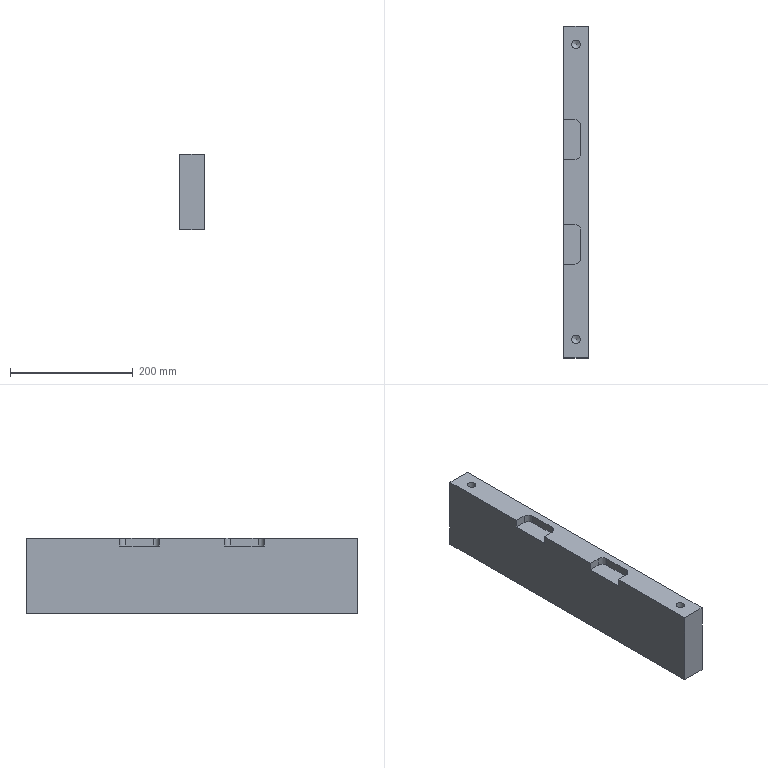Part | NX | features LIN_SOLID_COLOR 2 | 1 solid | 22 faces | box 40 x 540 x 123.5 mm | volume 2609030 mm3 | plane 14 | cylinder 6 | cone 2 | commonest cylinder face diameters 20 x4 14 x2
STEP:
#1=CARTESIAN_POINT('',(606.,270.,-106.5));
#2=VERTEX_POINT('',#1);
#3=CARTESIAN_POINT('',(566.,270.,-106.5));
#4=VERTEX_POINT('',#3);
#5=CARTESIAN_POINT('',(-164.,270.,-106.5));
#6=DIRECTION('',(1.,0.,0.));
#7=VECTOR('',#6,1000.);
#8=LINE('',#5,#7);
#9=EDGE_CURVE('',#2,#4,#8,.F.);
#10=ORIENTED_EDGE('',*,*,#9,.F.);
#11=CARTESIAN_POINT('',(606.,270.,-230.));
#12=VERTEX_POINT('',#11);
#13=CARTESIAN_POINT('',(606.,270.,-111.5));
#14=DIRECTION('',(0.,0.,-1.));
#15=VECTOR('',#14,1000.);
#16=LINE('',#13,#15);
#17=EDGE_CURVE('',#12,#2,#16,.F.);
#18=ORIENTED_EDGE('',*,*,#17,.F.);
#19=CARTESIAN_POINT('',(566.,270.,-230.));
#20=VERTEX_POINT('',#19);
#21=CARTESIAN_POINT('',(426.,270.,-230.));
#22=DIRECTION('',(1.,0.,0.));
#23=VECTOR('',#22,1000.);
#24=LINE('',#21,#23);
#25=EDGE_CURVE('',#12,#20,#24,.F.);
#26=ORIENTED_EDGE('',*,*,#25,.T.);
#27=CARTESIAN_POINT('',(566.,270.,-111.5));
#28=DIRECTION('',(0.,0.,-1.));
#29=VECTOR('',#28,1000.);
#30=LINE('',#27,#29);
#31=EDGE_CURVE('',#20,#4,#30,.F.);
#32=ORIENTED_EDGE('',*,*,#31,.T.);
#33=EDGE_LOOP('',(#10,#18,#26,#32));
#34=FACE_BOUND('',#33,.T.);
#35=CARTESIAN_POINT('',(426.,270.,-111.5));
#36=DIRECTION('',(0.,1.,0.));
#37=DIRECTION('',(0.,0.,1.));
#38=AXIS2_PLACEMENT_3D('',#35,#36,#37);
#39=PLANE('',#38);
#40=ADVANCED_FACE('',(#34),#39,.T.);
#41=CARTESIAN_POINT('',(566.,-270.,-230.));
#42=VERTEX_POINT('',#41);
#43=CARTESIAN_POINT('',(566.,0.,-230.));
#44=DIRECTION('',(0.,-1.,0.));
#45=VECTOR('',#44,1000.);
#46=LINE('',#43,#45);
#47=EDGE_CURVE('',#20,#42,#46,.T.);
#48=ORIENTED_EDGE('',*,*,#47,.F.);
#49=ORIENTED_EDGE('',*,*,#25,.F.);
#50=CARTESIAN_POINT('',(606.,-270.,-230.));
#51=VERTEX_POINT('',#50);
#52=CARTESIAN_POINT('',(606.,0.,-230.));
#53=DIRECTION('',(0.,-1.,0.));
#54=VECTOR('',#53,1000.);
#55=LINE('',#52,#54);
#56=EDGE_CURVE('',#12,#51,#55,.T.);
#57=ORIENTED_EDGE('',*,*,#56,.T.);
#58=CARTESIAN_POINT('',(426.,-270.,-230.));
#59=DIRECTION('',(1.,0.,0.));
#60=VECTOR('',#59,1000.);
#61=LINE('',#58,#60);
#62=EDGE_CURVE('',#51,#42,#61,.F.);
#63=ORIENTED_EDGE('',*,*,#62,.T.);
#64=EDGE_LOOP('',(#48,#49,#57,#63));
#65=FACE_BOUND('',#64,.T.);
#66=CARTESIAN_POINT('',(426.,0.,-230.));
#67=DIRECTION('',(0.,0.,1.));
#68=DIRECTION('',(-1.,0.,0.));
#69=AXIS2_PLACEMENT_3D('',#66,#67,#68);
#70=PLANE('',#69);
#71=ADVANCED_FACE('',(#65),#70,.F.);
#72=ORIENTED_EDGE('',*,*,#62,.F.);
#73=CARTESIAN_POINT('',(606.,-270.,-106.5));
#74=VERTEX_POINT('',#73);
#75=CARTESIAN_POINT('',(606.,-270.,-101.5));
#76=DIRECTION('',(0.,0.,-1.));
#77=VECTOR('',#76,1000.);
#78=LINE('',#75,#77);
#79=EDGE_CURVE('',#51,#74,#78,.F.);
#80=ORIENTED_EDGE('',*,*,#79,.T.);
#81=CARTESIAN_POINT('',(566.,-270.,-106.5));
#82=VERTEX_POINT('',#81);
#83=CARTESIAN_POINT('',(426.,-270.,-106.5));
#84=DIRECTION('',(1.,0.,0.));
#85=VECTOR('',#84,1000.);
#86=LINE('',#83,#85);
#87=EDGE_CURVE('',#74,#82,#86,.F.);
#88=ORIENTED_EDGE('',*,*,#87,.T.);
#89=CARTESIAN_POINT('',(566.,-270.,-101.5));
#90=DIRECTION('',(0.,0.,-1.));
#91=VECTOR('',#90,1000.);
#92=LINE('',#89,#91);
#93=EDGE_CURVE('',#42,#82,#92,.F.);
#94=ORIENTED_EDGE('',*,*,#93,.F.);
#95=EDGE_LOOP('',(#72,#80,#88,#94));
#96=FACE_BOUND('',#95,.T.);
#97=CARTESIAN_POINT('',(426.,-270.,-111.5));
#98=DIRECTION('',(0.,-1.,0.));
#99=DIRECTION('',(0.,0.,-1.));
#100=AXIS2_PLACEMENT_3D('',#97,#98,#99);
#101=PLANE('',#100);
#102=ADVANCED_FACE('',(#96),#101,.T.);
#103=CARTESIAN_POINT('',(566.,117.5,-106.5));
#104=VERTEX_POINT('',#103);
#105=CARTESIAN_POINT('',(566.,0.,-106.5));
#106=DIRECTION('',(0.,1.,0.));
#107=VECTOR('',#106,1000.);
#108=LINE('',#105,#107);
#109=EDGE_CURVE('',#104,#4,#108,.T.);
#110=ORIENTED_EDGE('',*,*,#109,.F.);
#111=CARTESIAN_POINT('',(584.,117.5,-106.5));
#112=VERTEX_POINT('',#111);
#113=CARTESIAN_POINT('',(-164.,117.5,-106.5));
#114=DIRECTION('',(1.,0.,0.));
#115=VECTOR('',#114,1000.);
#116=LINE('',#113,#115);
#117=EDGE_CURVE('',#104,#112,#116,.T.);
#118=ORIENTED_EDGE('',*,*,#117,.T.);
#119=CARTESIAN_POINT('',(594.,107.5,-106.5));
#120=VERTEX_POINT('',#119);
#121=CARTESIAN_POINT('',(584.,107.5,-106.5));
#122=DIRECTION('',(0.,0.,-1.));
#123=DIRECTION('',(-1.,0.,0.));
#124=AXIS2_PLACEMENT_3D('',#121,#122,#123);
#125=CIRCLE('',#124,10.);
#126=EDGE_CURVE('',#112,#120,#125,.T.);
#127=ORIENTED_EDGE('',*,*,#126,.T.);
#128=CARTESIAN_POINT('',(594.,63.,-106.5));
#129=VERTEX_POINT('',#128);
#130=CARTESIAN_POINT('',(594.,0.,-106.5));
#131=DIRECTION('',(0.,-1.,0.));
#132=VECTOR('',#131,1000.);
#133=LINE('',#130,#132);
#134=EDGE_CURVE('',#120,#129,#133,.T.);
#135=ORIENTED_EDGE('',*,*,#134,.T.);
#136=CARTESIAN_POINT('',(584.,53.,-106.5));
#137=VERTEX_POINT('',#136);
#138=CARTESIAN_POINT('',(584.,63.,-106.5));
#139=DIRECTION('',(0.,0.,-1.));
#140=DIRECTION('',(-1.,0.,0.));
#141=AXIS2_PLACEMENT_3D('',#138,#139,#140);
#142=CIRCLE('',#141,10.);
#143=EDGE_CURVE('',#129,#137,#142,.T.);
#144=ORIENTED_EDGE('',*,*,#143,.T.);
#145=CARTESIAN_POINT('',(566.,53.,-106.5));
#146=VERTEX_POINT('',#145);
#147=CARTESIAN_POINT('',(-164.,53.,-106.5));
#148=DIRECTION('',(-1.,0.,0.));
#149=VECTOR('',#148,1000.);
#150=LINE('',#147,#149);
#151=EDGE_CURVE('',#137,#146,#150,.T.);
#152=ORIENTED_EDGE('',*,*,#151,.T.);
#153=CARTESIAN_POINT('',(566.,-53.,-106.5));
#154=VERTEX_POINT('',#153);
#155=CARTESIAN_POINT('',(566.,0.,-106.5));
#156=DIRECTION('',(0.,1.,0.));
#157=VECTOR('',#156,1000.);
#158=LINE('',#155,#157);
#159=EDGE_CURVE('',#154,#146,#158,.T.);
#160=ORIENTED_EDGE('',*,*,#159,.F.);
#161=CARTESIAN_POINT('',(584.,-53.,-106.5));
#162=VERTEX_POINT('',#161);
#163=CARTESIAN_POINT('',(-164.,-53.,-106.5));
#164=DIRECTION('',(1.,0.,0.));
#165=VECTOR('',#164,1000.);
#166=LINE('',#163,#165);
#167=EDGE_CURVE('',#154,#162,#166,.T.);
#168=ORIENTED_EDGE('',*,*,#167,.T.);
#169=CARTESIAN_POINT('',(594.,-63.,-106.5));
#170=VERTEX_POINT('',#169);
#171=CARTESIAN_POINT('',(584.,-63.,-106.5));
#172=DIRECTION('',(0.,0.,-1.));
#173=DIRECTION('',(-1.,0.,0.));
#174=AXIS2_PLACEMENT_3D('',#171,#172,#173);
#175=CIRCLE('',#174,10.);
#176=EDGE_CURVE('',#162,#170,#175,.T.);
#177=ORIENTED_EDGE('',*,*,#176,.T.);
#178=CARTESIAN_POINT('',(594.,-107.5,-106.5));
#179=VERTEX_POINT('',#178);
#180=CARTESIAN_POINT('',(594.,0.,-106.5));
#181=DIRECTION('',(0.,-1.,0.));
#182=VECTOR('',#181,1000.);
#183=LINE('',#180,#182);
#184=EDGE_CURVE('',#170,#179,#183,.T.);
#185=ORIENTED_EDGE('',*,*,#184,.T.);
#186=CARTESIAN_POINT('',(584.,-117.5,-106.5));
#187=VERTEX_POINT('',#186);
#188=CARTESIAN_POINT('',(584.,-107.5,-106.5));
#189=DIRECTION('',(0.,0.,-1.));
#190=DIRECTION('',(-1.,0.,0.));
#191=AXIS2_PLACEMENT_3D('',#188,#189,#190);
#192=CIRCLE('',#191,10.);
#193=EDGE_CURVE('',#179,#187,#192,.T.);
#194=ORIENTED_EDGE('',*,*,#193,.T.);
#195=CARTESIAN_POINT('',(566.,-117.5,-106.5));
#196=VERTEX_POINT('',#195);
#197=CARTESIAN_POINT('',(-164.,-117.5,-106.5));
#198=DIRECTION('',(-1.,0.,0.));
#199=VECTOR('',#198,1000.);
#200=LINE('',#197,#199);
#201=EDGE_CURVE('',#187,#196,#200,.T.);
#202=ORIENTED_EDGE('',*,*,#201,.T.);
#203=CARTESIAN_POINT('',(566.,0.,-106.5));
#204=DIRECTION('',(0.,1.,0.));
#205=VECTOR('',#204,1000.);
#206=LINE('',#203,#205);
#207=EDGE_CURVE('',#82,#196,#206,.T.);
#208=ORIENTED_EDGE('',*,*,#207,.F.);
#209=ORIENTED_EDGE('',*,*,#87,.F.);
#210=CARTESIAN_POINT('',(606.,0.,-106.5));
#211=DIRECTION('',(0.,1.,0.));
#212=VECTOR('',#211,1000.);
#213=LINE('',#210,#212);
#214=EDGE_CURVE('',#74,#2,#213,.T.);
#215=ORIENTED_EDGE('',*,*,#214,.T.);
#216=ORIENTED_EDGE('',*,*,#9,.T.);
#217=EDGE_LOOP('',(#110,#118,#127,#135,#144,#152,#160,#168,#177,#185,#194,#202,#208,#209,#215,#216));
#218=FACE_BOUND('',#217,.T.);
#219=CARTESIAN_POINT('',(579.,240.,-106.5));
#220=VERTEX_POINT('',#219);
#221=CARTESIAN_POINT('',(586.,240.,-106.5));
#222=DIRECTION('',(0.,0.,-1.));
#223=DIRECTION('',(-1.,0.,0.));
#224=AXIS2_PLACEMENT_3D('',#221,#222,#223);
#225=CIRCLE('',#224,7.);
#226=EDGE_CURVE('',#220,#220,#225,.F.);
#227=ORIENTED_EDGE('',*,*,#226,.F.);
#228=EDGE_LOOP('',(#227));
#229=FACE_BOUND('',#228,.T.);
#230=CARTESIAN_POINT('',(579.,-240.,-106.5));
#231=VERTEX_POINT('',#230);
#232=CARTESIAN_POINT('',(586.,-240.,-106.5));
#233=DIRECTION('',(0.,0.,-1.));
#234=DIRECTION('',(-1.,0.,0.));
#235=AXIS2_PLACEMENT_3D('',#232,#233,#234);
#236=CIRCLE('',#235,7.);
#237=EDGE_CURVE('',#231,#231,#236,.F.);
#238=ORIENTED_EDGE('',*,*,#237,.F.);
#239=EDGE_LOOP('',(#238));
#240=FACE_BOUND('',#239,.T.);
#241=CARTESIAN_POINT('',(-164.,0.,-106.5));
#242=DIRECTION('',(0.,0.,-1.));
#243=DIRECTION('',(1.,0.,0.));
#244=AXIS2_PLACEMENT_3D('',#241,#242,#243);
#245=PLANE('',#244);
#246=ADVANCED_FACE('',(#218,#229,#240),#245,.F.);
#247=ORIENTED_EDGE('',*,*,#159,.T.);
#248=CARTESIAN_POINT('',(566.,53.,-119.5));
#249=VERTEX_POINT('',#248);
#250=CARTESIAN_POINT('',(566.,53.,-101.5));
#251=DIRECTION('',(0.,0.,-1.));
#252=VECTOR('',#251,1000.);
#253=LINE('',#250,#252);
#254=EDGE_CURVE('',#146,#249,#253,.T.);
#255=ORIENTED_EDGE('',*,*,#254,.T.);
#256=CARTESIAN_POINT('',(566.,117.5,-119.5));
#257=VERTEX_POINT('',#256);
#258=CARTESIAN_POINT('',(566.,0.,-119.5));
#259=DIRECTION('',(0.,1.,0.));
#260=VECTOR('',#259,1000.);
#261=LINE('',#258,#260);
#262=EDGE_CURVE('',#249,#257,#261,.T.);
#263=ORIENTED_EDGE('',*,*,#262,.T.);
#264=CARTESIAN_POINT('',(566.,117.5,-101.5));
#265=DIRECTION('',(0.,0.,1.));
#266=VECTOR('',#265,1000.);
#267=LINE('',#264,#266);
#268=EDGE_CURVE('',#257,#104,#267,.T.);
#269=ORIENTED_EDGE('',*,*,#268,.T.);
#270=ORIENTED_EDGE('',*,*,#109,.T.);
#271=ORIENTED_EDGE('',*,*,#31,.F.);
#272=ORIENTED_EDGE('',*,*,#47,.T.);
#273=ORIENTED_EDGE('',*,*,#93,.T.);
#274=ORIENTED_EDGE('',*,*,#207,.T.);
#275=CARTESIAN_POINT('',(566.,-117.5,-119.5));
#276=VERTEX_POINT('',#275);
#277=CARTESIAN_POINT('',(566.,-117.5,-101.5));
#278=DIRECTION('',(0.,0.,-1.));
#279=VECTOR('',#278,1000.);
#280=LINE('',#277,#279);
#281=EDGE_CURVE('',#196,#276,#280,.T.);
#282=ORIENTED_EDGE('',*,*,#281,.T.);
#283=CARTESIAN_POINT('',(566.,-53.,-119.5));
#284=VERTEX_POINT('',#283);
#285=CARTESIAN_POINT('',(566.,0.,-119.5));
#286=DIRECTION('',(0.,1.,0.));
#287=VECTOR('',#286,1000.);
#288=LINE('',#285,#287);
#289=EDGE_CURVE('',#276,#284,#288,.T.);
#290=ORIENTED_EDGE('',*,*,#289,.T.);
#291=CARTESIAN_POINT('',(566.,-53.,-101.5));
#292=DIRECTION('',(0.,0.,1.));
#293=VECTOR('',#292,1000.);
#294=LINE('',#291,#293);
#295=EDGE_CURVE('',#284,#154,#294,.T.);
#296=ORIENTED_EDGE('',*,*,#295,.T.);
#297=EDGE_LOOP('',(#247,#255,#263,#269,#270,#271,#272,#273,#274,#282,#290,#296));
#298=FACE_BOUND('',#297,.T.);
#299=CARTESIAN_POINT('',(566.,0.,-101.5));
#300=DIRECTION('',(1.,0.,0.));
#301=DIRECTION('',(0.,0.,1.));
#302=AXIS2_PLACEMENT_3D('',#299,#300,#301);
#303=PLANE('',#302);
#304=ADVANCED_FACE('',(#298),#303,.F.);
#305=ORIENTED_EDGE('',*,*,#79,.F.);
#306=ORIENTED_EDGE('',*,*,#56,.F.);
#307=ORIENTED_EDGE('',*,*,#17,.T.);
#308=ORIENTED_EDGE('',*,*,#214,.F.);
#309=EDGE_LOOP('',(#305,#306,#307,#308));
#310=FACE_BOUND('',#309,.T.);
#311=CARTESIAN_POINT('',(606.,0.,-101.5));
#312=DIRECTION('',(1.,0.,0.));
#313=DIRECTION('',(0.,0.,1.));
#314=AXIS2_PLACEMENT_3D('',#311,#312,#313);
#315=PLANE('',#314);
#316=ADVANCED_FACE('',(#310),#315,.T.);
#317=CARTESIAN_POINT('',(593.,-240.,-146.5));
#318=VERTEX_POINT('',#317);
#319=CARTESIAN_POINT('',(586.,-240.,-146.5));
#320=DIRECTION('',(0.,0.,1.));
#321=DIRECTION('',(1.,0.,0.));
#322=AXIS2_PLACEMENT_3D('',#319,#320,#321);
#323=CIRCLE('',#322,7.);
#324=EDGE_CURVE('',#318,#318,#323,.F.);
#325=ORIENTED_EDGE('',*,*,#324,.T.);
#326=EDGE_LOOP('',(#325));
#327=FACE_BOUND('',#326,.T.);
#328=ORIENTED_EDGE('',*,*,#237,.T.);
#329=EDGE_LOOP('',(#328));
#330=FACE_BOUND('',#329,.T.);
#331=CARTESIAN_POINT('',(586.,-240.,-106.4));
#332=DIRECTION('',(0.,0.,-1.));
#333=DIRECTION('',(-1.,0.,0.));
#334=AXIS2_PLACEMENT_3D('',#331,#332,#333);
#335=CYLINDRICAL_SURFACE('',#334,7.);
#336=ADVANCED_FACE('',(#327,#330),#335,.F.);
#337=ORIENTED_EDGE('',*,*,#324,.F.);
#338=EDGE_LOOP('',(#337));
#339=FACE_BOUND('',#338,.T.);
#340=CARTESIAN_POINT('',(586.,-240.,-150.541));
#341=VERTEX_POINT('',#340);
#342=VERTEX_LOOP('',#341);
#343=FACE_BOUND('',#342,.T.);
#344=CARTESIAN_POINT('',(586.,-240.,-150.541));
#345=DIRECTION('',(0.,0.,1.));
#346=DIRECTION('',(-1.,0.,0.));
#347=AXIS2_PLACEMENT_3D('',#344,#345,#346);
#348=CONICAL_SURFACE('',#347,0.,1.047);
#349=ADVANCED_FACE('',(#339,#343),#348,.F.);
#350=CARTESIAN_POINT('',(593.,240.,-146.5));
#351=VERTEX_POINT('',#350);
#352=CARTESIAN_POINT('',(586.,240.,-146.5));
#353=DIRECTION('',(0.,0.,1.));
#354=DIRECTION('',(1.,0.,0.));
#355=AXIS2_PLACEMENT_3D('',#352,#353,#354);
#356=CIRCLE('',#355,7.);
#357=EDGE_CURVE('',#351,#351,#356,.F.);
#358=ORIENTED_EDGE('',*,*,#357,.T.);
#359=EDGE_LOOP('',(#358));
#360=FACE_BOUND('',#359,.T.);
#361=ORIENTED_EDGE('',*,*,#226,.T.);
#362=EDGE_LOOP('',(#361));
#363=FACE_BOUND('',#362,.T.);
#364=CARTESIAN_POINT('',(586.,240.,-106.4));
#365=DIRECTION('',(0.,0.,-1.));
#366=DIRECTION('',(-1.,0.,0.));
#367=AXIS2_PLACEMENT_3D('',#364,#365,#366);
#368=CYLINDRICAL_SURFACE('',#367,7.);
#369=ADVANCED_FACE('',(#360,#363),#368,.F.);
#370=ORIENTED_EDGE('',*,*,#357,.F.);
#371=EDGE_LOOP('',(#370));
#372=FACE_BOUND('',#371,.T.);
#373=CARTESIAN_POINT('',(586.,240.,-150.541));
#374=VERTEX_POINT('',#373);
#375=VERTEX_LOOP('',#374);
#376=FACE_BOUND('',#375,.T.);
#377=CARTESIAN_POINT('',(586.,240.,-150.541));
#378=DIRECTION('',(0.,0.,1.));
#379=DIRECTION('',(-1.,0.,0.));
#380=AXIS2_PLACEMENT_3D('',#377,#378,#379);
#381=CONICAL_SURFACE('',#380,0.,1.047);
#382=ADVANCED_FACE('',(#372,#376),#381,.F.);
#383=CARTESIAN_POINT('',(594.,-63.,-119.5));
#384=VERTEX_POINT('',#383);
#385=CARTESIAN_POINT('',(594.,-63.,-112.5));
#386=DIRECTION('',(0.,0.,1.));
#387=VECTOR('',#386,1000.);
#388=LINE('',#385,#387);
#389=EDGE_CURVE('',#170,#384,#388,.F.);
#390=ORIENTED_EDGE('',*,*,#389,.T.);
#391=CARTESIAN_POINT('',(594.,-107.5,-119.5));
#392=VERTEX_POINT('',#391);
#393=CARTESIAN_POINT('',(594.,-103.,-119.5));
#394=DIRECTION('',(0.,1.,0.));
#395=VECTOR('',#394,1000.);
#396=LINE('',#393,#395);
#397=EDGE_CURVE('',#384,#392,#396,.F.);
#398=ORIENTED_EDGE('',*,*,#397,.T.);
#399=CARTESIAN_POINT('',(594.,-107.5,-112.5));
#400=DIRECTION('',(0.,0.,1.));
#401=VECTOR('',#400,1000.);
#402=LINE('',#399,#401);
#403=EDGE_CURVE('',#179,#392,#402,.F.);
#404=ORIENTED_EDGE('',*,*,#403,.F.);
#405=ORIENTED_EDGE('',*,*,#184,.F.);
#406=EDGE_LOOP('',(#390,#398,#404,#405));
#407=FACE_BOUND('',#406,.T.);
#408=CARTESIAN_POINT('',(594.,-103.,-112.5));
#409=DIRECTION('',(1.,0.,0.));
#410=DIRECTION('',(0.,0.,-1.));
#411=AXIS2_PLACEMENT_3D('',#408,#409,#410);
#412=PLANE('',#411);
#413=ADVANCED_FACE('',(#407),#412,.F.);
#414=CARTESIAN_POINT('',(584.,-53.,-119.5));
#415=VERTEX_POINT('',#414);
#416=CARTESIAN_POINT('',(584.,-53.,-119.5));
#417=DIRECTION('',(0.,0.,1.));
#418=VECTOR('',#417,1000.);
#419=LINE('',#416,#418);
#420=EDGE_CURVE('',#415,#162,#419,.T.);
#421=ORIENTED_EDGE('',*,*,#420,.F.);
#422=CARTESIAN_POINT('',(584.,-63.,-119.5));
#423=DIRECTION('',(0.,0.,-1.));
#424=DIRECTION('',(-1.,0.,0.));
#425=AXIS2_PLACEMENT_3D('',#422,#423,#424);
#426=CIRCLE('',#425,10.);
#427=EDGE_CURVE('',#384,#415,#426,.F.);
#428=ORIENTED_EDGE('',*,*,#427,.F.);
#429=ORIENTED_EDGE('',*,*,#389,.F.);
#430=ORIENTED_EDGE('',*,*,#176,.F.);
#431=EDGE_LOOP('',(#421,#428,#429,#430));
#432=FACE_BOUND('',#431,.T.);
#433=CARTESIAN_POINT('',(584.,-63.,-112.5));
#434=DIRECTION('',(0.,0.,1.));
#435=DIRECTION('',(1.,0.,0.));
#436=AXIS2_PLACEMENT_3D('',#433,#434,#435);
#437=CYLINDRICAL_SURFACE('',#436,10.);
#438=ADVANCED_FACE('',(#432),#437,.F.);
#439=ORIENTED_EDGE('',*,*,#403,.T.);
#440=CARTESIAN_POINT('',(584.,-117.5,-119.5));
#441=VERTEX_POINT('',#440);
#442=CARTESIAN_POINT('',(584.,-107.5,-119.5));
#443=DIRECTION('',(0.,0.,-1.));
#444=DIRECTION('',(-1.,0.,0.));
#445=AXIS2_PLACEMENT_3D('',#442,#443,#444);
#446=CIRCLE('',#445,10.);
#447=EDGE_CURVE('',#392,#441,#446,.T.);
#448=ORIENTED_EDGE('',*,*,#447,.T.);
#449=CARTESIAN_POINT('',(584.,-117.5,-112.5));
#450=DIRECTION('',(0.,0.,1.));
#451=VECTOR('',#450,1000.);
#452=LINE('',#449,#451);
#453=EDGE_CURVE('',#187,#441,#452,.F.);
#454=ORIENTED_EDGE('',*,*,#453,.F.);
#455=ORIENTED_EDGE('',*,*,#193,.F.);
#456=EDGE_LOOP('',(#439,#448,#454,#455));
#457=FACE_BOUND('',#456,.T.);
#458=CARTESIAN_POINT('',(584.,-107.5,-112.5));
#459=DIRECTION('',(0.,0.,1.));
#460=DIRECTION('',(1.,0.,0.));
#461=AXIS2_PLACEMENT_3D('',#458,#459,#460);
#462=CYLINDRICAL_SURFACE('',#461,10.);
#463=ADVANCED_FACE('',(#457),#462,.F.);
#464=ORIENTED_EDGE('',*,*,#295,.F.);
#465=CARTESIAN_POINT('',(563.,-53.,-119.5));
#466=DIRECTION('',(-1.,0.,0.));
#467=VECTOR('',#466,1000.);
#468=LINE('',#465,#467);
#469=EDGE_CURVE('',#284,#415,#468,.F.);
#470=ORIENTED_EDGE('',*,*,#469,.T.);
#471=ORIENTED_EDGE('',*,*,#420,.T.);
#472=ORIENTED_EDGE('',*,*,#167,.F.);
#473=EDGE_LOOP('',(#464,#470,#471,#472));
#474=FACE_BOUND('',#473,.T.);
#475=CARTESIAN_POINT('',(563.,-53.,-119.5));
#476=DIRECTION('',(0.,1.,0.));
#477=DIRECTION('',(0.,0.,1.));
#478=AXIS2_PLACEMENT_3D('',#475,#476,#477);
#479=PLANE('',#478);
#480=ADVANCED_FACE('',(#474),#479,.F.);
#481=CARTESIAN_POINT('',(579.5,-117.5,-119.5));
#482=DIRECTION('',(1.,0.,0.));
#483=VECTOR('',#482,1000.);
#484=LINE('',#481,#483);
#485=EDGE_CURVE('',#276,#441,#484,.T.);
#486=ORIENTED_EDGE('',*,*,#485,.T.);
#487=ORIENTED_EDGE('',*,*,#447,.F.);
#488=ORIENTED_EDGE('',*,*,#397,.F.);
#489=ORIENTED_EDGE('',*,*,#427,.T.);
#490=ORIENTED_EDGE('',*,*,#469,.F.);
#491=ORIENTED_EDGE('',*,*,#289,.F.);
#492=EDGE_LOOP('',(#486,#487,#488,#489,#490,#491));
#493=FACE_BOUND('',#492,.T.);
#494=CARTESIAN_POINT('',(563.,-67.,-119.5));
#495=DIRECTION('',(0.,0.,-1.));
#496=DIRECTION('',(-1.,0.,0.));
#497=AXIS2_PLACEMENT_3D('',#494,#495,#496);
#498=PLANE('',#497);
#499=ADVANCED_FACE('',(#493),#498,.F.);
#500=ORIENTED_EDGE('',*,*,#453,.T.);
#501=ORIENTED_EDGE('',*,*,#485,.F.);
#502=ORIENTED_EDGE('',*,*,#281,.F.);
#503=ORIENTED_EDGE('',*,*,#201,.F.);
#504=EDGE_LOOP('',(#500,#501,#502,#503));
#505=FACE_BOUND('',#504,.T.);
#506=CARTESIAN_POINT('',(579.5,-117.5,-112.5));
#507=DIRECTION('',(0.,-1.,0.));
#508=DIRECTION('',(0.,0.,-1.));
#509=AXIS2_PLACEMENT_3D('',#506,#507,#508);
#510=PLANE('',#509);
#511=ADVANCED_FACE('',(#505),#510,.F.);
#512=CARTESIAN_POINT('',(594.,107.5,-119.5));
#513=VERTEX_POINT('',#512);
#514=CARTESIAN_POINT('',(594.,107.5,-112.5));
#515=DIRECTION('',(0.,0.,-1.));
#516=VECTOR('',#515,1000.);
#517=LINE('',#514,#516);
#518=EDGE_CURVE('',#120,#513,#517,.T.);
#519=ORIENTED_EDGE('',*,*,#518,.T.);
#520=CARTESIAN_POINT('',(594.,63.,-119.5));
#521=VERTEX_POINT('',#520);
#522=CARTESIAN_POINT('',(594.,-103.,-119.5));
#523=DIRECTION('',(0.,1.,0.));
#524=VECTOR('',#523,1000.);
#525=LINE('',#522,#524);
#526=EDGE_CURVE('',#513,#521,#525,.F.);
#527=ORIENTED_EDGE('',*,*,#526,.T.);
#528=CARTESIAN_POINT('',(594.,63.,-112.5));
#529=DIRECTION('',(0.,0.,-1.));
#530=VECTOR('',#529,1000.);
#531=LINE('',#528,#530);
#532=EDGE_CURVE('',#521,#129,#531,.F.);
#533=ORIENTED_EDGE('',*,*,#532,.T.);
#534=ORIENTED_EDGE('',*,*,#134,.F.);
#535=EDGE_LOOP('',(#519,#527,#533,#534));
#536=FACE_BOUND('',#535,.T.);
#537=CARTESIAN_POINT('',(594.,-103.,-112.5));
#538=DIRECTION('',(1.,0.,0.));
#539=DIRECTION('',(0.,0.,-1.));
#540=AXIS2_PLACEMENT_3D('',#537,#538,#539);
#541=PLANE('',#540);
#542=ADVANCED_FACE('',(#536),#541,.F.);
#543=CARTESIAN_POINT('',(584.,117.5,-119.5));
#544=VERTEX_POINT('',#543);
#545=CARTESIAN_POINT('',(584.,117.5,-112.5));
#546=DIRECTION('',(0.,0.,-1.));
#547=VECTOR('',#546,1000.);
#548=LINE('',#545,#547);
#549=EDGE_CURVE('',#544,#112,#548,.F.);
#550=ORIENTED_EDGE('',*,*,#549,.F.);
#551=CARTESIAN_POINT('',(584.,107.5,-119.5));
#552=DIRECTION('',(0.,0.,-1.));
#553=DIRECTION('',(-1.,0.,0.));
#554=AXIS2_PLACEMENT_3D('',#551,#552,#553);
#555=CIRCLE('',#554,10.);
#556=EDGE_CURVE('',#513,#544,#555,.F.);
#557=ORIENTED_EDGE('',*,*,#556,.F.);
#558=ORIENTED_EDGE('',*,*,#518,.F.);
#559=ORIENTED_EDGE('',*,*,#126,.F.);
#560=EDGE_LOOP('',(#550,#557,#558,#559));
#561=FACE_BOUND('',#560,.T.);
#562=CARTESIAN_POINT('',(584.,107.5,-112.5));
#563=DIRECTION('',(0.,0.,-1.));
#564=DIRECTION('',(-1.,0.,0.));
#565=AXIS2_PLACEMENT_3D('',#562,#563,#564);
#566=CYLINDRICAL_SURFACE('',#565,10.);
#567=ADVANCED_FACE('',(#561),#566,.F.);
#568=ORIENTED_EDGE('',*,*,#532,.F.);
#569=CARTESIAN_POINT('',(584.,53.,-119.5));
#570=VERTEX_POINT('',#569);
#571=CARTESIAN_POINT('',(584.,63.,-119.5));
#572=DIRECTION('',(0.,0.,-1.));
#573=DIRECTION('',(-1.,0.,0.));
#574=AXIS2_PLACEMENT_3D('',#571,#572,#573);
#575=CIRCLE('',#574,10.);
#576=EDGE_CURVE('',#570,#521,#575,.F.);
#577=ORIENTED_EDGE('',*,*,#576,.F.);
#578=CARTESIAN_POINT('',(584.,53.,-119.5));
#579=DIRECTION('',(0.,0.,-1.));
#580=VECTOR('',#579,1000.);
#581=LINE('',#578,#580);
#582=EDGE_CURVE('',#137,#570,#581,.T.);
#583=ORIENTED_EDGE('',*,*,#582,.F.);
#584=ORIENTED_EDGE('',*,*,#143,.F.);
#585=EDGE_LOOP('',(#568,#577,#583,#584));
#586=FACE_BOUND('',#585,.T.);
#587=CARTESIAN_POINT('',(584.,63.,-112.5));
#588=DIRECTION('',(0.,0.,-1.));
#589=DIRECTION('',(-1.,0.,0.));
#590=AXIS2_PLACEMENT_3D('',#587,#588,#589);
#591=CYLINDRICAL_SURFACE('',#590,10.);
#592=ADVANCED_FACE('',(#586),#591,.F.);
#593=ORIENTED_EDGE('',*,*,#582,.T.);
#594=CARTESIAN_POINT('',(563.,53.,-119.5));
#595=DIRECTION('',(1.,0.,0.));
#596=VECTOR('',#595,1000.);
#597=LINE('',#594,#596);
#598=EDGE_CURVE('',#570,#249,#597,.F.);
#599=ORIENTED_EDGE('',*,*,#598,.T.);
#600=ORIENTED_EDGE('',*,*,#254,.F.);
#601=ORIENTED_EDGE('',*,*,#151,.F.);
#602=EDGE_LOOP('',(#593,#599,#600,#601));
#603=FACE_BOUND('',#602,.T.);
#604=CARTESIAN_POINT('',(563.,53.,-119.5));
#605=DIRECTION('',(0.,-1.,0.));
#606=DIRECTION('',(0.,0.,-1.));
#607=AXIS2_PLACEMENT_3D('',#604,#605,#606);
#608=PLANE('',#607);
#609=ADVANCED_FACE('',(#603),#608,.F.);
#610=ORIENTED_EDGE('',*,*,#268,.F.);
#611=CARTESIAN_POINT('',(545.5,117.5,-119.5));
#612=DIRECTION('',(-1.,0.,0.));
#613=VECTOR('',#612,1000.);
#614=LINE('',#611,#613);
#615=EDGE_CURVE('',#257,#544,#614,.F.);
#616=ORIENTED_EDGE('',*,*,#615,.T.);
#617=ORIENTED_EDGE('',*,*,#549,.T.);
#618=ORIENTED_EDGE('',*,*,#117,.F.);
#619=EDGE_LOOP('',(#610,#616,#617,#618));
#620=FACE_BOUND('',#619,.T.);
#621=CARTESIAN_POINT('',(545.5,117.5,-112.5));
#622=DIRECTION('',(0.,1.,0.));
#623=DIRECTION('',(0.,0.,1.));
#624=AXIS2_PLACEMENT_3D('',#621,#622,#623);
#625=PLANE('',#624);
#626=ADVANCED_FACE('',(#620),#625,.F.);
#627=ORIENTED_EDGE('',*,*,#598,.F.);
#628=ORIENTED_EDGE('',*,*,#576,.T.);
#629=ORIENTED_EDGE('',*,*,#526,.F.);
#630=ORIENTED_EDGE('',*,*,#556,.T.);
#631=ORIENTED_EDGE('',*,*,#615,.F.);
#632=ORIENTED_EDGE('',*,*,#262,.F.);
#633=EDGE_LOOP('',(#627,#628,#629,#630,#631,#632));
#634=FACE_BOUND('',#633,.T.);
#635=CARTESIAN_POINT('',(563.,67.,-119.5));
#636=DIRECTION('',(0.,0.,-1.));
#637=DIRECTION('',(-1.,0.,0.));
#638=AXIS2_PLACEMENT_3D('',#635,#636,#637);
#639=PLANE('',#638);
#640=ADVANCED_FACE('',(#634),#639,.F.);
#641=CLOSED_SHELL('',(#40,#71,#102,#246,#304,#316,#336,#349,#369,#382,#413,#438,#463,#480,#499,#511,#542,#567,#592,#609,#626,#640));
#642=MANIFOLD_SOLID_BREP('',#641);
#643=(LENGTH_UNIT()NAMED_UNIT(*)SI_UNIT(.MILLI.,.METRE.));
#644=UNCERTAINTY_MEASURE_WITH_UNIT(LENGTH_MEASURE(0.00001),#643,'','');
#645=(NAMED_UNIT(*)PLANE_ANGLE_UNIT()SI_UNIT($,.RADIAN.));
#646=(NAMED_UNIT(*)SI_UNIT($,.STERADIAN.)SOLID_ANGLE_UNIT());
#647=(GEOMETRIC_REPRESENTATION_CONTEXT(3)GLOBAL_UNCERTAINTY_ASSIGNED_CONTEXT((#644))GLOBAL_UNIT_ASSIGNED_CONTEXT((#643,#645,#646))REPRESENTATION_CONTEXT('',''));
#648=ADVANCED_BREP_SHAPE_REPRESENTATION('',(#642),#647);